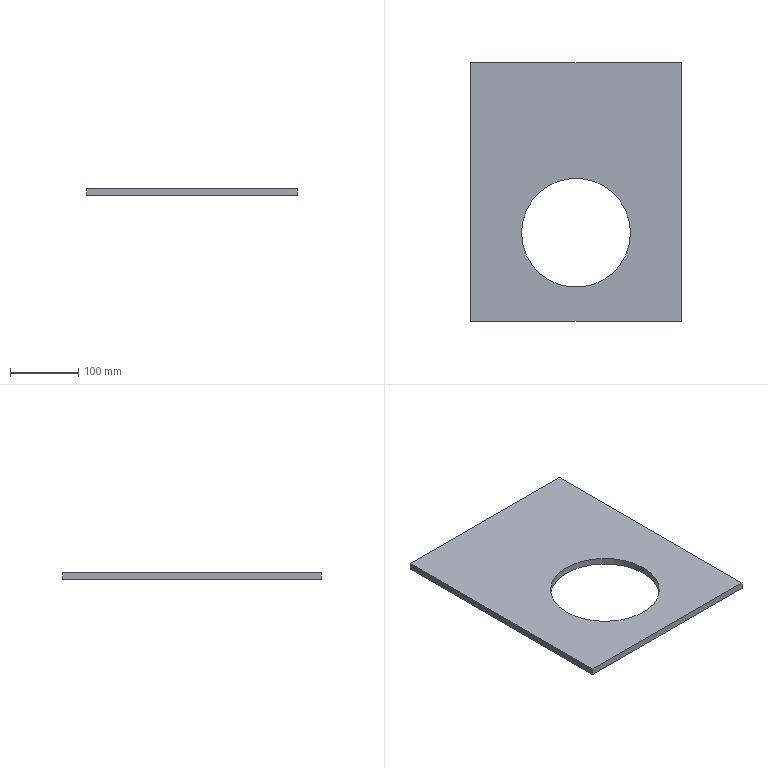Part | STEP file | 机台DoorPlate开Hole-单元二 | 1 solid | 8 faces | box 310 x 380 x 10 mm | volume 976938 mm3 | plane 6 | cylinder 2 | commonest cylinder face diameters 160 x2
STEP:
#1=CARTESIAN_POINT('',(0.,0.,0.));
#2=DIRECTION('',(0.,0.,1.));
#3=DIRECTION('',(1.,0.,0.));
#4=AXIS2_PLACEMENT_3D('',#1,#2,#3);
#5=CARTESIAN_POINT('',(80.,-60.,0.));
#6=VERTEX_POINT('',#5);
#7=CARTESIAN_POINT('',(80.,-60.,10.));
#8=VERTEX_POINT('',#7);
#9=CARTESIAN_POINT('',(80.,-60.,0.));
#10=DIRECTION('',(0.,0.,1.));
#11=VECTOR('',#10,1.);
#12=LINE('',#9,#11);
#13=CARTESIAN_POINT('',(0.,-60.,0.));
#14=DIRECTION('',(0.,0.,1.));
#15=DIRECTION('',(1.,0.,0.));
#16=AXIS2_PLACEMENT_3D('',#13,#14,#15);
#17=CYLINDRICAL_SURFACE('',#16,80.);
#18=CARTESIAN_POINT('',(6.283,0.));
#19=DIRECTION('',(0.,1.));
#20=VECTOR('',#19,1.);
#21=LINE('',#18,#20);
#22=(GEOMETRIC_REPRESENTATION_CONTEXT(2)PARAMETRIC_REPRESENTATION_CONTEXT()REPRESENTATION_CONTEXT('',''));
#23=DEFINITIONAL_REPRESENTATION('',(#21),#22);
#24=PCURVE('',#17,#23);
#25=CARTESIAN_POINT('',(0.,-60.,0.));
#26=DIRECTION('',(0.,0.,1.));
#27=DIRECTION('',(1.,0.,0.));
#28=AXIS2_PLACEMENT_3D('',#25,#26,#27);
#29=CYLINDRICAL_SURFACE('',#28,80.);
#30=CARTESIAN_POINT('',(0.,0.));
#31=DIRECTION('',(0.,1.));
#32=VECTOR('',#31,1.);
#33=LINE('',#30,#32);
#34=(GEOMETRIC_REPRESENTATION_CONTEXT(2)PARAMETRIC_REPRESENTATION_CONTEXT()REPRESENTATION_CONTEXT('',''));
#35=DEFINITIONAL_REPRESENTATION('',(#33),#34);
#36=PCURVE('',#29,#35);
#37=SURFACE_CURVE('',#12,(#24,#36),.PCURVE_S1.);
#38=EDGE_CURVE('',#6,#8,#37,.T.);
#39=ORIENTED_EDGE('',*,*,#38,.T.);
#40=CARTESIAN_POINT('',(-80.,-60.,10.));
#41=VERTEX_POINT('',#40);
#42=CARTESIAN_POINT('',(0.,-60.,10.));
#43=DIRECTION('',(0.,0.,1.));
#44=DIRECTION('',(1.,0.,0.));
#45=AXIS2_PLACEMENT_3D('',#42,#43,#44);
#46=CIRCLE('',#45,80.);
#47=CARTESIAN_POINT('',(0.,10.));
#48=DIRECTION('',(1.,0.));
#49=VECTOR('',#48,1.);
#50=LINE('',#47,#49);
#51=(GEOMETRIC_REPRESENTATION_CONTEXT(2)PARAMETRIC_REPRESENTATION_CONTEXT()REPRESENTATION_CONTEXT('',''));
#52=DEFINITIONAL_REPRESENTATION('',(#50),#51);
#53=PCURVE('',#17,#52);
#54=CARTESIAN_POINT('',(0.,0.,10.));
#55=DIRECTION('',(0.,0.,-1.));
#56=DIRECTION('',(-1.,0.,0.));
#57=AXIS2_PLACEMENT_3D('',#54,#55,#56);
#58=PLANE('',#57);
#59=CARTESIAN_POINT('',(-80.,-60.));
#60=CARTESIAN_POINT('',(-80.,78.564));
#61=CARTESIAN_POINT('',(40.,9.282));
#62=CARTESIAN_POINT('',(160.,-60.));
#63=CARTESIAN_POINT('',(40.,-129.282));
#64=CARTESIAN_POINT('',(-80.,-198.564));
#65=CARTESIAN_POINT('',(-80.,-60.));
#66=(BOUNDED_CURVE()B_SPLINE_CURVE(2,(#59,#60,#61,#62,#63,#64,#65),.UNSPECIFIED.,.T.,.F.)B_SPLINE_CURVE_WITH_KNOTS((1,2,2,2,2,1),(-2.094,0.,2.094,4.189,6.283,8.378),.UNSPECIFIED.)CURVE()GEOMETRIC_REPRESENTATION_ITEM()RATIONAL_B_SPLINE_CURVE((1.,0.5,1.,0.5,1.,0.5,1.))REPRESENTATION_ITEM(''));
#67=(GEOMETRIC_REPRESENTATION_CONTEXT(2)PARAMETRIC_REPRESENTATION_CONTEXT()REPRESENTATION_CONTEXT('',''));
#68=DEFINITIONAL_REPRESENTATION('',(#66),#67);
#69=PCURVE('',#58,#68);
#70=SURFACE_CURVE('',#46,(#53,#69),.PCURVE_S1.);
#71=EDGE_CURVE('',#41,#8,#70,.T.);
#72=ORIENTED_EDGE('',*,*,#71,.F.);
#73=CARTESIAN_POINT('',(-80.,-60.,0.));
#74=VERTEX_POINT('',#73);
#75=CARTESIAN_POINT('',(-80.,-60.,0.));
#76=DIRECTION('',(0.,0.,1.));
#77=VECTOR('',#76,1.);
#78=LINE('',#75,#77);
#79=CARTESIAN_POINT('',(3.142,0.));
#80=DIRECTION('',(0.,1.));
#81=VECTOR('',#80,1.);
#82=LINE('',#79,#81);
#83=(GEOMETRIC_REPRESENTATION_CONTEXT(2)PARAMETRIC_REPRESENTATION_CONTEXT()REPRESENTATION_CONTEXT('',''));
#84=DEFINITIONAL_REPRESENTATION('',(#82),#83);
#85=PCURVE('',#17,#84);
#86=CARTESIAN_POINT('',(3.142,0.));
#87=DIRECTION('',(0.,1.));
#88=VECTOR('',#87,1.);
#89=LINE('',#86,#88);
#90=(GEOMETRIC_REPRESENTATION_CONTEXT(2)PARAMETRIC_REPRESENTATION_CONTEXT()REPRESENTATION_CONTEXT('',''));
#91=DEFINITIONAL_REPRESENTATION('',(#89),#90);
#92=PCURVE('',#29,#91);
#93=SURFACE_CURVE('',#78,(#85,#92),.PCURVE_S1.);
#94=EDGE_CURVE('',#74,#41,#93,.T.);
#95=ORIENTED_EDGE('',*,*,#94,.F.);
#96=CARTESIAN_POINT('',(0.,-60.,0.));
#97=DIRECTION('',(0.,0.,1.));
#98=DIRECTION('',(1.,0.,0.));
#99=AXIS2_PLACEMENT_3D('',#96,#97,#98);
#100=CIRCLE('',#99,80.);
#101=CARTESIAN_POINT('',(0.,0.));
#102=DIRECTION('',(1.,0.));
#103=VECTOR('',#102,1.);
#104=LINE('',#101,#103);
#105=(GEOMETRIC_REPRESENTATION_CONTEXT(2)PARAMETRIC_REPRESENTATION_CONTEXT()REPRESENTATION_CONTEXT('',''));
#106=DEFINITIONAL_REPRESENTATION('',(#104),#105);
#107=PCURVE('',#17,#106);
#108=CARTESIAN_POINT('',(0.,0.,0.));
#109=DIRECTION('',(0.,0.,-1.));
#110=DIRECTION('',(-1.,0.,0.));
#111=AXIS2_PLACEMENT_3D('',#108,#109,#110);
#112=PLANE('',#111);
#113=CARTESIAN_POINT('',(-80.,-60.));
#114=CARTESIAN_POINT('',(-80.,78.564));
#115=CARTESIAN_POINT('',(40.,9.282));
#116=CARTESIAN_POINT('',(160.,-60.));
#117=CARTESIAN_POINT('',(40.,-129.282));
#118=CARTESIAN_POINT('',(-80.,-198.564));
#119=CARTESIAN_POINT('',(-80.,-60.));
#120=(BOUNDED_CURVE()B_SPLINE_CURVE(2,(#113,#114,#115,#116,#117,#118,#119),.UNSPECIFIED.,.T.,.F.)B_SPLINE_CURVE_WITH_KNOTS((1,2,2,2,2,1),(-2.094,0.,2.094,4.189,6.283,8.378),.UNSPECIFIED.)CURVE()GEOMETRIC_REPRESENTATION_ITEM()RATIONAL_B_SPLINE_CURVE((1.,0.5,1.,0.5,1.,0.5,1.))REPRESENTATION_ITEM(''));
#121=(GEOMETRIC_REPRESENTATION_CONTEXT(2)PARAMETRIC_REPRESENTATION_CONTEXT()REPRESENTATION_CONTEXT('',''));
#122=DEFINITIONAL_REPRESENTATION('',(#120),#121);
#123=PCURVE('',#112,#122);
#124=SURFACE_CURVE('',#100,(#107,#123),.PCURVE_S1.);
#125=EDGE_CURVE('',#74,#6,#124,.T.);
#126=ORIENTED_EDGE('',*,*,#125,.T.);
#127=EDGE_LOOP('',(#39,#72,#95,#126));
#128=FACE_BOUND('',#127,.F.);
#129=ADVANCED_FACE('',(#128),#17,.F.);
#130=CARTESIAN_POINT('',(155.,-190.,0.));
#131=VERTEX_POINT('',#130);
#132=CARTESIAN_POINT('',(155.,190.,0.));
#133=VERTEX_POINT('',#132);
#134=CARTESIAN_POINT('',(155.,-190.,0.));
#135=DIRECTION('',(0.,1.,0.));
#136=VECTOR('',#135,1.);
#137=LINE('',#134,#136);
#138=CARTESIAN_POINT('',(155.,-190.,10.));
#139=DIRECTION('',(-1.,0.,0.));
#140=DIRECTION('',(0.,0.,1.));
#141=AXIS2_PLACEMENT_3D('',#138,#139,#140);
#142=PLANE('',#141);
#143=CARTESIAN_POINT('',(-10.,0.));
#144=DIRECTION('',(0.,1.));
#145=VECTOR('',#144,1.);
#146=LINE('',#143,#145);
#147=(GEOMETRIC_REPRESENTATION_CONTEXT(2)PARAMETRIC_REPRESENTATION_CONTEXT()REPRESENTATION_CONTEXT('',''));
#148=DEFINITIONAL_REPRESENTATION('',(#146),#147);
#149=PCURVE('',#142,#148);
#150=CARTESIAN_POINT('',(-155.,-190.));
#151=DIRECTION('',(0.,1.));
#152=VECTOR('',#151,1.);
#153=LINE('',#150,#152);
#154=(GEOMETRIC_REPRESENTATION_CONTEXT(2)PARAMETRIC_REPRESENTATION_CONTEXT()REPRESENTATION_CONTEXT('',''));
#155=DEFINITIONAL_REPRESENTATION('',(#153),#154);
#156=PCURVE('',#112,#155);
#157=SURFACE_CURVE('',#137,(#149,#156),.PCURVE_S1.);
#158=EDGE_CURVE('',#131,#133,#157,.T.);
#159=ORIENTED_EDGE('',*,*,#158,.T.);
#160=CARTESIAN_POINT('',(155.,190.,10.));
#161=VERTEX_POINT('',#160);
#162=CARTESIAN_POINT('',(155.,190.,10.));
#163=DIRECTION('',(0.,0.,-1.));
#164=VECTOR('',#163,1.);
#165=LINE('',#162,#164);
#166=CARTESIAN_POINT('',(0.,380.));
#167=DIRECTION('',(-1.,0.));
#168=VECTOR('',#167,1.);
#169=LINE('',#166,#168);
#170=(GEOMETRIC_REPRESENTATION_CONTEXT(2)PARAMETRIC_REPRESENTATION_CONTEXT()REPRESENTATION_CONTEXT('',''));
#171=DEFINITIONAL_REPRESENTATION('',(#169),#170);
#172=PCURVE('',#142,#171);
#173=CARTESIAN_POINT('',(-155.,190.,10.));
#174=DIRECTION('',(0.,-1.,0.));
#175=DIRECTION('',(0.,0.,-1.));
#176=AXIS2_PLACEMENT_3D('',#173,#174,#175);
#177=PLANE('',#176);
#178=CARTESIAN_POINT('',(0.,310.));
#179=DIRECTION('',(1.,0.));
#180=VECTOR('',#179,1.);
#181=LINE('',#178,#180);
#182=(GEOMETRIC_REPRESENTATION_CONTEXT(2)PARAMETRIC_REPRESENTATION_CONTEXT()REPRESENTATION_CONTEXT('',''));
#183=DEFINITIONAL_REPRESENTATION('',(#181),#182);
#184=PCURVE('',#177,#183);
#185=SURFACE_CURVE('',#165,(#172,#184),.PCURVE_S1.);
#186=EDGE_CURVE('',#161,#133,#185,.T.);
#187=ORIENTED_EDGE('',*,*,#186,.F.);
#188=CARTESIAN_POINT('',(155.,-190.,10.));
#189=VERTEX_POINT('',#188);
#190=CARTESIAN_POINT('',(155.,-190.,10.));
#191=DIRECTION('',(0.,1.,0.));
#192=VECTOR('',#191,1.);
#193=LINE('',#190,#192);
#194=CARTESIAN_POINT('',(0.,0.));
#195=DIRECTION('',(0.,1.));
#196=VECTOR('',#195,1.);
#197=LINE('',#194,#196);
#198=(GEOMETRIC_REPRESENTATION_CONTEXT(2)PARAMETRIC_REPRESENTATION_CONTEXT()REPRESENTATION_CONTEXT('',''));
#199=DEFINITIONAL_REPRESENTATION('',(#197),#198);
#200=PCURVE('',#142,#199);
#201=CARTESIAN_POINT('',(-155.,-190.));
#202=DIRECTION('',(0.,1.));
#203=VECTOR('',#202,1.);
#204=LINE('',#201,#203);
#205=(GEOMETRIC_REPRESENTATION_CONTEXT(2)PARAMETRIC_REPRESENTATION_CONTEXT()REPRESENTATION_CONTEXT('',''));
#206=DEFINITIONAL_REPRESENTATION('',(#204),#205);
#207=PCURVE('',#58,#206);
#208=SURFACE_CURVE('',#193,(#200,#207),.PCURVE_S1.);
#209=EDGE_CURVE('',#189,#161,#208,.T.);
#210=ORIENTED_EDGE('',*,*,#209,.F.);
#211=CARTESIAN_POINT('',(155.,-190.,10.));
#212=DIRECTION('',(0.,0.,-1.));
#213=VECTOR('',#212,1.);
#214=LINE('',#211,#213);
#215=CARTESIAN_POINT('',(0.,0.));
#216=DIRECTION('',(-1.,0.));
#217=VECTOR('',#216,1.);
#218=LINE('',#215,#217);
#219=(GEOMETRIC_REPRESENTATION_CONTEXT(2)PARAMETRIC_REPRESENTATION_CONTEXT()REPRESENTATION_CONTEXT('',''));
#220=DEFINITIONAL_REPRESENTATION('',(#218),#219);
#221=PCURVE('',#142,#220);
#222=CARTESIAN_POINT('',(-155.,-190.,10.));
#223=DIRECTION('',(0.,1.,0.));
#224=DIRECTION('',(0.,0.,1.));
#225=AXIS2_PLACEMENT_3D('',#222,#223,#224);
#226=PLANE('',#225);
#227=CARTESIAN_POINT('',(0.,310.));
#228=DIRECTION('',(-1.,0.));
#229=VECTOR('',#228,1.);
#230=LINE('',#227,#229);
#231=(GEOMETRIC_REPRESENTATION_CONTEXT(2)PARAMETRIC_REPRESENTATION_CONTEXT()REPRESENTATION_CONTEXT('',''));
#232=DEFINITIONAL_REPRESENTATION('',(#230),#231);
#233=PCURVE('',#226,#232);
#234=SURFACE_CURVE('',#214,(#221,#233),.PCURVE_S1.);
#235=EDGE_CURVE('',#189,#131,#234,.T.);
#236=ORIENTED_EDGE('',*,*,#235,.T.);
#237=EDGE_LOOP('',(#159,#187,#210,#236));
#238=FACE_BOUND('',#237,.T.);
#239=ADVANCED_FACE('',(#238),#142,.F.);
#240=CARTESIAN_POINT('',(-155.,190.,0.));
#241=VERTEX_POINT('',#240);
#242=CARTESIAN_POINT('',(-155.,190.,0.));
#243=DIRECTION('',(-1.,0.,0.));
#244=VECTOR('',#243,1.);
#245=LINE('',#242,#244);
#246=CARTESIAN_POINT('',(10.,0.));
#247=DIRECTION('',(0.,-1.));
#248=VECTOR('',#247,1.);
#249=LINE('',#246,#248);
#250=(GEOMETRIC_REPRESENTATION_CONTEXT(2)PARAMETRIC_REPRESENTATION_CONTEXT()REPRESENTATION_CONTEXT('',''));
#251=DEFINITIONAL_REPRESENTATION('',(#249),#250);
#252=PCURVE('',#177,#251);
#253=CARTESIAN_POINT('',(155.,190.));
#254=DIRECTION('',(1.,0.));
#255=VECTOR('',#254,1.);
#256=LINE('',#253,#255);
#257=(GEOMETRIC_REPRESENTATION_CONTEXT(2)PARAMETRIC_REPRESENTATION_CONTEXT()REPRESENTATION_CONTEXT('',''));
#258=DEFINITIONAL_REPRESENTATION('',(#256),#257);
#259=PCURVE('',#112,#258);
#260=SURFACE_CURVE('',#245,(#252,#259),.PCURVE_S1.);
#261=EDGE_CURVE('',#133,#241,#260,.T.);
#262=ORIENTED_EDGE('',*,*,#261,.T.);
#263=CARTESIAN_POINT('',(-155.,190.,10.));
#264=VERTEX_POINT('',#263);
#265=CARTESIAN_POINT('',(-155.,190.,10.));
#266=DIRECTION('',(0.,0.,-1.));
#267=VECTOR('',#266,1.);
#268=LINE('',#265,#267);
#269=CARTESIAN_POINT('',(0.,0.));
#270=DIRECTION('',(1.,0.));
#271=VECTOR('',#270,1.);
#272=LINE('',#269,#271);
#273=(GEOMETRIC_REPRESENTATION_CONTEXT(2)PARAMETRIC_REPRESENTATION_CONTEXT()REPRESENTATION_CONTEXT('',''));
#274=DEFINITIONAL_REPRESENTATION('',(#272),#273);
#275=PCURVE('',#177,#274);
#276=CARTESIAN_POINT('',(-155.,-190.,10.));
#277=DIRECTION('',(1.,0.,0.));
#278=DIRECTION('',(0.,0.,-1.));
#279=AXIS2_PLACEMENT_3D('',#276,#277,#278);
#280=PLANE('',#279);
#281=CARTESIAN_POINT('',(0.,380.));
#282=DIRECTION('',(1.,0.));
#283=VECTOR('',#282,1.);
#284=LINE('',#281,#283);
#285=(GEOMETRIC_REPRESENTATION_CONTEXT(2)PARAMETRIC_REPRESENTATION_CONTEXT()REPRESENTATION_CONTEXT('',''));
#286=DEFINITIONAL_REPRESENTATION('',(#284),#285);
#287=PCURVE('',#280,#286);
#288=SURFACE_CURVE('',#268,(#275,#287),.PCURVE_S1.);
#289=EDGE_CURVE('',#264,#241,#288,.T.);
#290=ORIENTED_EDGE('',*,*,#289,.F.);
#291=CARTESIAN_POINT('',(-155.,190.,10.));
#292=DIRECTION('',(-1.,0.,0.));
#293=VECTOR('',#292,1.);
#294=LINE('',#291,#293);
#295=CARTESIAN_POINT('',(0.,0.));
#296=DIRECTION('',(0.,-1.));
#297=VECTOR('',#296,1.);
#298=LINE('',#295,#297);
#299=(GEOMETRIC_REPRESENTATION_CONTEXT(2)PARAMETRIC_REPRESENTATION_CONTEXT()REPRESENTATION_CONTEXT('',''));
#300=DEFINITIONAL_REPRESENTATION('',(#298),#299);
#301=PCURVE('',#177,#300);
#302=CARTESIAN_POINT('',(155.,190.));
#303=DIRECTION('',(1.,0.));
#304=VECTOR('',#303,1.);
#305=LINE('',#302,#304);
#306=(GEOMETRIC_REPRESENTATION_CONTEXT(2)PARAMETRIC_REPRESENTATION_CONTEXT()REPRESENTATION_CONTEXT('',''));
#307=DEFINITIONAL_REPRESENTATION('',(#305),#306);
#308=PCURVE('',#58,#307);
#309=SURFACE_CURVE('',#294,(#301,#308),.PCURVE_S1.);
#310=EDGE_CURVE('',#161,#264,#309,.T.);
#311=ORIENTED_EDGE('',*,*,#310,.F.);
#312=ORIENTED_EDGE('',*,*,#186,.T.);
#313=EDGE_LOOP('',(#262,#290,#311,#312));
#314=FACE_BOUND('',#313,.T.);
#315=ADVANCED_FACE('',(#314),#177,.F.);
#316=CARTESIAN_POINT('',(-155.,-190.,0.));
#317=VERTEX_POINT('',#316);
#318=CARTESIAN_POINT('',(-155.,-190.,0.));
#319=DIRECTION('',(0.,-1.,0.));
#320=VECTOR('',#319,1.);
#321=LINE('',#318,#320);
#322=CARTESIAN_POINT('',(10.,0.));
#323=DIRECTION('',(0.,-1.));
#324=VECTOR('',#323,1.);
#325=LINE('',#322,#324);
#326=(GEOMETRIC_REPRESENTATION_CONTEXT(2)PARAMETRIC_REPRESENTATION_CONTEXT()REPRESENTATION_CONTEXT('',''));
#327=DEFINITIONAL_REPRESENTATION('',(#325),#326);
#328=PCURVE('',#280,#327);
#329=CARTESIAN_POINT('',(155.,-190.));
#330=DIRECTION('',(0.,-1.));
#331=VECTOR('',#330,1.);
#332=LINE('',#329,#331);
#333=(GEOMETRIC_REPRESENTATION_CONTEXT(2)PARAMETRIC_REPRESENTATION_CONTEXT()REPRESENTATION_CONTEXT('',''));
#334=DEFINITIONAL_REPRESENTATION('',(#332),#333);
#335=PCURVE('',#112,#334);
#336=SURFACE_CURVE('',#321,(#328,#335),.PCURVE_S1.);
#337=EDGE_CURVE('',#241,#317,#336,.T.);
#338=ORIENTED_EDGE('',*,*,#337,.T.);
#339=CARTESIAN_POINT('',(-155.,-190.,10.));
#340=VERTEX_POINT('',#339);
#341=CARTESIAN_POINT('',(-155.,-190.,10.));
#342=DIRECTION('',(0.,0.,-1.));
#343=VECTOR('',#342,1.);
#344=LINE('',#341,#343);
#345=CARTESIAN_POINT('',(0.,0.));
#346=DIRECTION('',(1.,0.));
#347=VECTOR('',#346,1.);
#348=LINE('',#345,#347);
#349=(GEOMETRIC_REPRESENTATION_CONTEXT(2)PARAMETRIC_REPRESENTATION_CONTEXT()REPRESENTATION_CONTEXT('',''));
#350=DEFINITIONAL_REPRESENTATION('',(#348),#349);
#351=PCURVE('',#280,#350);
#352=CARTESIAN_POINT('',(0.,0.));
#353=DIRECTION('',(-1.,0.));
#354=VECTOR('',#353,1.);
#355=LINE('',#352,#354);
#356=(GEOMETRIC_REPRESENTATION_CONTEXT(2)PARAMETRIC_REPRESENTATION_CONTEXT()REPRESENTATION_CONTEXT('',''));
#357=DEFINITIONAL_REPRESENTATION('',(#355),#356);
#358=PCURVE('',#226,#357);
#359=SURFACE_CURVE('',#344,(#351,#358),.PCURVE_S1.);
#360=EDGE_CURVE('',#340,#317,#359,.T.);
#361=ORIENTED_EDGE('',*,*,#360,.F.);
#362=CARTESIAN_POINT('',(-155.,-190.,10.));
#363=DIRECTION('',(0.,-1.,0.));
#364=VECTOR('',#363,1.);
#365=LINE('',#362,#364);
#366=CARTESIAN_POINT('',(0.,0.));
#367=DIRECTION('',(0.,-1.));
#368=VECTOR('',#367,1.);
#369=LINE('',#366,#368);
#370=(GEOMETRIC_REPRESENTATION_CONTEXT(2)PARAMETRIC_REPRESENTATION_CONTEXT()REPRESENTATION_CONTEXT('',''));
#371=DEFINITIONAL_REPRESENTATION('',(#369),#370);
#372=PCURVE('',#280,#371);
#373=CARTESIAN_POINT('',(155.,-190.));
#374=DIRECTION('',(0.,-1.));
#375=VECTOR('',#374,1.);
#376=LINE('',#373,#375);
#377=(GEOMETRIC_REPRESENTATION_CONTEXT(2)PARAMETRIC_REPRESENTATION_CONTEXT()REPRESENTATION_CONTEXT('',''));
#378=DEFINITIONAL_REPRESENTATION('',(#376),#377);
#379=PCURVE('',#58,#378);
#380=SURFACE_CURVE('',#365,(#372,#379),.PCURVE_S1.);
#381=EDGE_CURVE('',#264,#340,#380,.T.);
#382=ORIENTED_EDGE('',*,*,#381,.F.);
#383=ORIENTED_EDGE('',*,*,#289,.T.);
#384=EDGE_LOOP('',(#338,#361,#382,#383));
#385=FACE_BOUND('',#384,.T.);
#386=ADVANCED_FACE('',(#385),#280,.F.);
#387=CARTESIAN_POINT('',(-155.,-190.,0.));
#388=DIRECTION('',(1.,0.,0.));
#389=VECTOR('',#388,1.);
#390=LINE('',#387,#389);
#391=CARTESIAN_POINT('',(-10.,0.));
#392=DIRECTION('',(0.,1.));
#393=VECTOR('',#392,1.);
#394=LINE('',#391,#393);
#395=(GEOMETRIC_REPRESENTATION_CONTEXT(2)PARAMETRIC_REPRESENTATION_CONTEXT()REPRESENTATION_CONTEXT('',''));
#396=DEFINITIONAL_REPRESENTATION('',(#394),#395);
#397=PCURVE('',#226,#396);
#398=CARTESIAN_POINT('',(155.,-190.));
#399=DIRECTION('',(-1.,0.));
#400=VECTOR('',#399,1.);
#401=LINE('',#398,#400);
#402=(GEOMETRIC_REPRESENTATION_CONTEXT(2)PARAMETRIC_REPRESENTATION_CONTEXT()REPRESENTATION_CONTEXT('',''));
#403=DEFINITIONAL_REPRESENTATION('',(#401),#402);
#404=PCURVE('',#112,#403);
#405=SURFACE_CURVE('',#390,(#397,#404),.PCURVE_S1.);
#406=EDGE_CURVE('',#317,#131,#405,.T.);
#407=ORIENTED_EDGE('',*,*,#406,.T.);
#408=ORIENTED_EDGE('',*,*,#235,.F.);
#409=CARTESIAN_POINT('',(-155.,-190.,10.));
#410=DIRECTION('',(1.,0.,0.));
#411=VECTOR('',#410,1.);
#412=LINE('',#409,#411);
#413=CARTESIAN_POINT('',(0.,0.));
#414=DIRECTION('',(0.,1.));
#415=VECTOR('',#414,1.);
#416=LINE('',#413,#415);
#417=(GEOMETRIC_REPRESENTATION_CONTEXT(2)PARAMETRIC_REPRESENTATION_CONTEXT()REPRESENTATION_CONTEXT('',''));
#418=DEFINITIONAL_REPRESENTATION('',(#416),#417);
#419=PCURVE('',#226,#418);
#420=CARTESIAN_POINT('',(155.,-190.));
#421=DIRECTION('',(-1.,0.));
#422=VECTOR('',#421,1.);
#423=LINE('',#420,#422);
#424=(GEOMETRIC_REPRESENTATION_CONTEXT(2)PARAMETRIC_REPRESENTATION_CONTEXT()REPRESENTATION_CONTEXT('',''));
#425=DEFINITIONAL_REPRESENTATION('',(#423),#424);
#426=PCURVE('',#58,#425);
#427=SURFACE_CURVE('',#412,(#419,#426),.PCURVE_S1.);
#428=EDGE_CURVE('',#340,#189,#427,.T.);
#429=ORIENTED_EDGE('',*,*,#428,.F.);
#430=ORIENTED_EDGE('',*,*,#360,.T.);
#431=EDGE_LOOP('',(#407,#408,#429,#430));
#432=FACE_BOUND('',#431,.T.);
#433=ADVANCED_FACE('',(#432),#226,.F.);
#434=CARTESIAN_POINT('',(0.,-60.,10.));
#435=DIRECTION('',(0.,0.,1.));
#436=DIRECTION('',(1.,0.,0.));
#437=AXIS2_PLACEMENT_3D('',#434,#435,#436);
#438=CIRCLE('',#437,80.);
#439=CARTESIAN_POINT('',(-80.,-60.));
#440=CARTESIAN_POINT('',(-80.,78.564));
#441=CARTESIAN_POINT('',(40.,9.282));
#442=CARTESIAN_POINT('',(160.,-60.));
#443=CARTESIAN_POINT('',(40.,-129.282));
#444=CARTESIAN_POINT('',(-80.,-198.564));
#445=CARTESIAN_POINT('',(-80.,-60.));
#446=(BOUNDED_CURVE()B_SPLINE_CURVE(2,(#439,#440,#441,#442,#443,#444,#445),.UNSPECIFIED.,.T.,.F.)B_SPLINE_CURVE_WITH_KNOTS((1,2,2,2,2,1),(-2.094,0.,2.094,4.189,6.283,8.378),.UNSPECIFIED.)CURVE()GEOMETRIC_REPRESENTATION_ITEM()RATIONAL_B_SPLINE_CURVE((1.,0.5,1.,0.5,1.,0.5,1.))REPRESENTATION_ITEM(''));
#447=(GEOMETRIC_REPRESENTATION_CONTEXT(2)PARAMETRIC_REPRESENTATION_CONTEXT()REPRESENTATION_CONTEXT('',''));
#448=DEFINITIONAL_REPRESENTATION('',(#446),#447);
#449=PCURVE('',#58,#448);
#450=CARTESIAN_POINT('',(0.,10.));
#451=DIRECTION('',(1.,0.));
#452=VECTOR('',#451,1.);
#453=LINE('',#450,#452);
#454=(GEOMETRIC_REPRESENTATION_CONTEXT(2)PARAMETRIC_REPRESENTATION_CONTEXT()REPRESENTATION_CONTEXT('',''));
#455=DEFINITIONAL_REPRESENTATION('',(#453),#454);
#456=PCURVE('',#29,#455);
#457=SURFACE_CURVE('',#438,(#449,#456),.PCURVE_S1.);
#458=EDGE_CURVE('',#8,#41,#457,.T.);
#459=ORIENTED_EDGE('',*,*,#458,.F.);
#460=ORIENTED_EDGE('',*,*,#71,.F.);
#461=EDGE_LOOP('',(#459,#460));
#462=FACE_BOUND('',#461,.T.);
#463=ORIENTED_EDGE('',*,*,#209,.T.);
#464=ORIENTED_EDGE('',*,*,#310,.T.);
#465=ORIENTED_EDGE('',*,*,#381,.T.);
#466=ORIENTED_EDGE('',*,*,#428,.T.);
#467=EDGE_LOOP('',(#463,#464,#465,#466));
#468=FACE_BOUND('',#467,.T.);
#469=ADVANCED_FACE('',(#462,#468),#58,.F.);
#470=CARTESIAN_POINT('',(0.,-60.,0.));
#471=DIRECTION('',(0.,0.,1.));
#472=DIRECTION('',(1.,0.,0.));
#473=AXIS2_PLACEMENT_3D('',#470,#471,#472);
#474=CIRCLE('',#473,80.);
#475=CARTESIAN_POINT('',(-80.,-60.));
#476=CARTESIAN_POINT('',(-80.,78.564));
#477=CARTESIAN_POINT('',(40.,9.282));
#478=CARTESIAN_POINT('',(160.,-60.));
#479=CARTESIAN_POINT('',(40.,-129.282));
#480=CARTESIAN_POINT('',(-80.,-198.564));
#481=CARTESIAN_POINT('',(-80.,-60.));
#482=(BOUNDED_CURVE()B_SPLINE_CURVE(2,(#475,#476,#477,#478,#479,#480,#481),.UNSPECIFIED.,.T.,.F.)B_SPLINE_CURVE_WITH_KNOTS((1,2,2,2,2,1),(-2.094,0.,2.094,4.189,6.283,8.378),.UNSPECIFIED.)CURVE()GEOMETRIC_REPRESENTATION_ITEM()RATIONAL_B_SPLINE_CURVE((1.,0.5,1.,0.5,1.,0.5,1.))REPRESENTATION_ITEM(''));
#483=(GEOMETRIC_REPRESENTATION_CONTEXT(2)PARAMETRIC_REPRESENTATION_CONTEXT()REPRESENTATION_CONTEXT('',''));
#484=DEFINITIONAL_REPRESENTATION('',(#482),#483);
#485=PCURVE('',#112,#484);
#486=CARTESIAN_POINT('',(0.,0.));
#487=DIRECTION('',(1.,0.));
#488=VECTOR('',#487,1.);
#489=LINE('',#486,#488);
#490=(GEOMETRIC_REPRESENTATION_CONTEXT(2)PARAMETRIC_REPRESENTATION_CONTEXT()REPRESENTATION_CONTEXT('',''));
#491=DEFINITIONAL_REPRESENTATION('',(#489),#490);
#492=PCURVE('',#29,#491);
#493=SURFACE_CURVE('',#474,(#485,#492),.PCURVE_S1.);
#494=EDGE_CURVE('',#6,#74,#493,.T.);
#495=ORIENTED_EDGE('',*,*,#494,.T.);
#496=ORIENTED_EDGE('',*,*,#125,.T.);
#497=EDGE_LOOP('',(#495,#496));
#498=FACE_BOUND('',#497,.T.);
#499=ORIENTED_EDGE('',*,*,#158,.F.);
#500=ORIENTED_EDGE('',*,*,#406,.F.);
#501=ORIENTED_EDGE('',*,*,#337,.F.);
#502=ORIENTED_EDGE('',*,*,#261,.F.);
#503=EDGE_LOOP('',(#499,#500,#501,#502));
#504=FACE_BOUND('',#503,.T.);
#505=ADVANCED_FACE('',(#498,#504),#112,.T.);
#506=ORIENTED_EDGE('',*,*,#458,.F.);
#507=ORIENTED_EDGE('',*,*,#38,.F.);
#508=ORIENTED_EDGE('',*,*,#494,.T.);
#509=ORIENTED_EDGE('',*,*,#94,.T.);
#510=EDGE_LOOP('',(#506,#507,#508,#509));
#511=FACE_BOUND('',#510,.F.);
#512=ADVANCED_FACE('',(#511),#29,.F.);
#513=CLOSED_SHELL('',(#129,#239,#315,#386,#433,#469,#505,#512));
#514=MANIFOLD_SOLID_BREP('',#513);
#515=(LENGTH_UNIT()NAMED_UNIT(*)SI_UNIT(.MILLI.,.METRE.));
#516=UNCERTAINTY_MEASURE_WITH_UNIT(LENGTH_MEASURE(0.0000001),#515,'','');
#517=(NAMED_UNIT(*)PLANE_ANGLE_UNIT()SI_UNIT($,.RADIAN.));
#518=(NAMED_UNIT(*)SI_UNIT($,.STERADIAN.)SOLID_ANGLE_UNIT());
#519=(GEOMETRIC_REPRESENTATION_CONTEXT(3)GLOBAL_UNCERTAINTY_ASSIGNED_CONTEXT((#516))GLOBAL_UNIT_ASSIGNED_CONTEXT((#515,#517,#518))REPRESENTATION_CONTEXT('',''));
#520=ADVANCED_BREP_SHAPE_REPRESENTATION('',(#4,#514),#519);